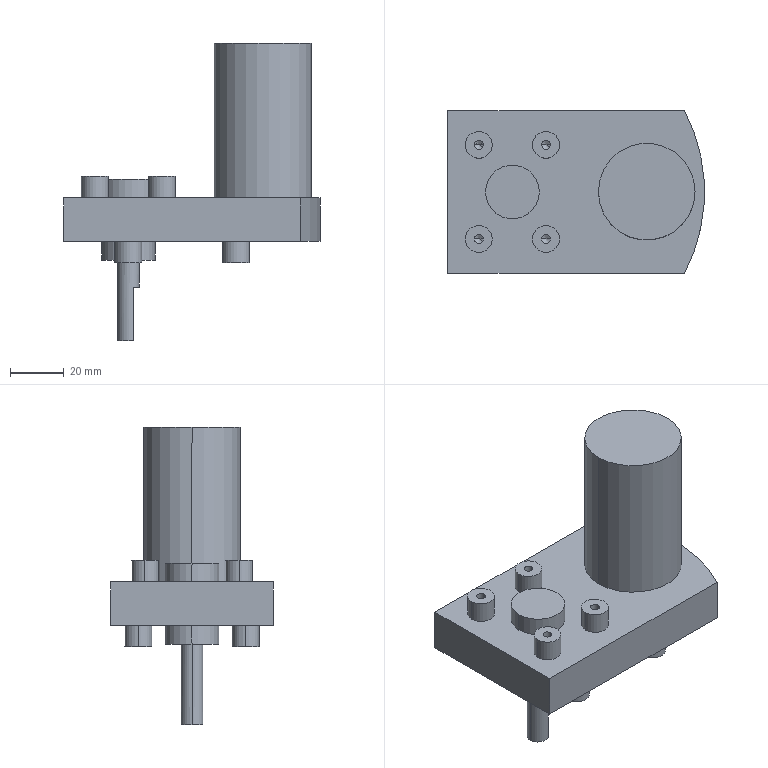Part | SolidWorks | features BaseBody 1 | 1 solid | 76 faces | box 95.5 x 60.5 x 110.8 mm | volume 160005 mm3 | cylinder 41 | plane 19 | cone 16 | commonest cylinder face diameters 3.3 x16 10 x16 20 x4 8 x2 36 x2 129.508 x1